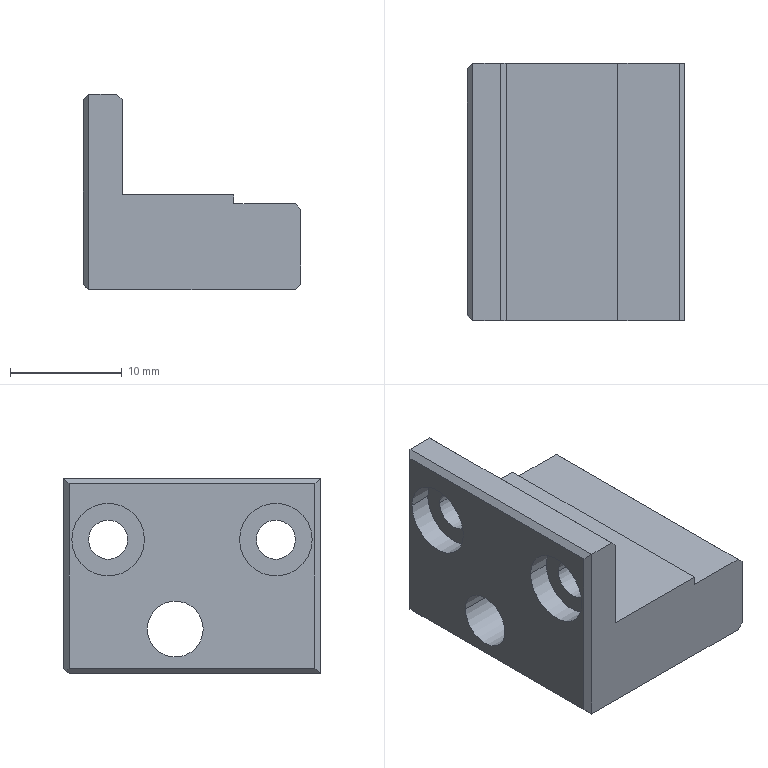Part | NX | 1 solid | 30 faces | box 19.5 x 23 x 17.5 mm | volume 3861 mm3 | plane 20 | cylinder 10 | commonest cylinder face diameters 3.5 x4 6.5 x4 5 x2
STEP:
#1=CARTESIAN_POINT('',(14.,5.5,-9.8));
#2=VERTEX_POINT('',#1);
#3=CARTESIAN_POINT('',(14.,28.5,-9.8));
#4=VERTEX_POINT('',#3);
#5=CARTESIAN_POINT('',(14.,0.,-9.8));
#6=DIRECTION('',(0.,1.,0.));
#7=VECTOR('',#6,1000.);
#8=LINE('',#5,#7);
#9=EDGE_CURVE('',#2,#4,#8,.T.);
#10=ORIENTED_EDGE('',*,*,#9,.F.);
#11=CARTESIAN_POINT('',(19.5,5.5,-9.8));
#12=VERTEX_POINT('',#11);
#13=CARTESIAN_POINT('',(0.,5.5,-9.8));
#14=DIRECTION('',(1.,0.,0.));
#15=VECTOR('',#14,1000.);
#16=LINE('',#13,#15);
#17=EDGE_CURVE('',#2,#12,#16,.T.);
#18=ORIENTED_EDGE('',*,*,#17,.T.);
#19=CARTESIAN_POINT('',(19.5,28.5,-9.8));
#20=VERTEX_POINT('',#19);
#21=CARTESIAN_POINT('',(19.5,14.5,-9.8));
#22=DIRECTION('',(0.,-1.,0.));
#23=VECTOR('',#22,1000.);
#24=LINE('',#21,#23);
#25=EDGE_CURVE('',#20,#12,#24,.T.);
#26=ORIENTED_EDGE('',*,*,#25,.F.);
#27=CARTESIAN_POINT('',(0.,28.5,-9.8));
#28=DIRECTION('',(1.,0.,0.));
#29=VECTOR('',#28,1000.);
#30=LINE('',#27,#29);
#31=EDGE_CURVE('',#4,#20,#30,.T.);
#32=ORIENTED_EDGE('',*,*,#31,.F.);
#33=EDGE_LOOP('',(#10,#18,#26,#32));
#34=FACE_BOUND('',#33,.T.);
#35=CARTESIAN_POINT('',(14.,14.5,-9.8));
#36=DIRECTION('',(0.,0.,1.));
#37=DIRECTION('',(1.,0.,0.));
#38=AXIS2_PLACEMENT_3D('',#35,#36,#37);
#39=PLANE('',#38);
#40=ADVANCED_FACE('',(#34),#39,.T.);
#41=CARTESIAN_POINT('',(2.5,21.25,-5.5));
#42=VERTEX_POINT('',#41);
#43=CARTESIAN_POINT('',(2.5,27.75,-5.5));
#44=VERTEX_POINT('',#43);
#45=CARTESIAN_POINT('',(2.5,24.5,-5.5));
#46=DIRECTION('',(-1.,0.,0.));
#47=DIRECTION('',(0.,1.,0.));
#48=AXIS2_PLACEMENT_3D('',#45,#46,#47);
#49=CIRCLE('',#48,3.25);
#50=EDGE_CURVE('',#42,#44,#49,.T.);
#51=ORIENTED_EDGE('',*,*,#50,.T.);
#52=CARTESIAN_POINT('',(2.5,24.5,-5.5));
#53=DIRECTION('',(-1.,0.,0.));
#54=DIRECTION('',(0.,1.,0.));
#55=AXIS2_PLACEMENT_3D('',#52,#53,#54);
#56=CIRCLE('',#55,3.25);
#57=EDGE_CURVE('',#44,#42,#56,.T.);
#58=ORIENTED_EDGE('',*,*,#57,.T.);
#59=EDGE_LOOP('',(#51,#58));
#60=FACE_BOUND('',#59,.T.);
#61=CARTESIAN_POINT('',(2.5,22.75,-5.5));
#62=VERTEX_POINT('',#61);
#63=CARTESIAN_POINT('',(2.5,26.25,-5.5));
#64=VERTEX_POINT('',#63);
#65=CARTESIAN_POINT('',(2.5,24.5,-5.5));
#66=DIRECTION('',(-1.,0.,0.));
#67=DIRECTION('',(0.,1.,0.));
#68=AXIS2_PLACEMENT_3D('',#65,#66,#67);
#69=CIRCLE('',#68,1.75);
#70=EDGE_CURVE('',#62,#64,#69,.T.);
#71=ORIENTED_EDGE('',*,*,#70,.F.);
#72=CARTESIAN_POINT('',(2.5,24.5,-5.5));
#73=DIRECTION('',(-1.,0.,0.));
#74=DIRECTION('',(0.,1.,0.));
#75=AXIS2_PLACEMENT_3D('',#72,#73,#74);
#76=CIRCLE('',#75,1.75);
#77=EDGE_CURVE('',#64,#62,#76,.T.);
#78=ORIENTED_EDGE('',*,*,#77,.F.);
#79=EDGE_LOOP('',(#71,#78));
#80=FACE_BOUND('',#79,.T.);
#81=CARTESIAN_POINT('',(2.5,24.5,-5.5));
#82=DIRECTION('',(-1.,0.,0.));
#83=DIRECTION('',(0.,0.,1.));
#84=AXIS2_PLACEMENT_3D('',#81,#82,#83);
#85=PLANE('',#84);
#86=ADVANCED_FACE('',(#60,#80),#85,.T.);
#87=CARTESIAN_POINT('',(1.,28.,-17.5));
#88=VERTEX_POINT('',#87);
#89=CARTESIAN_POINT('',(19.5,28.,-17.5));
#90=VERTEX_POINT('',#89);
#91=CARTESIAN_POINT('',(0.,28.,-17.5));
#92=DIRECTION('',(1.,0.,0.));
#93=VECTOR('',#92,1000.);
#94=LINE('',#91,#93);
#95=EDGE_CURVE('',#88,#90,#94,.T.);
#96=ORIENTED_EDGE('',*,*,#95,.F.);
#97=CARTESIAN_POINT('',(0.75,28.25,-17.25));
#98=VERTEX_POINT('',#97);
#99=CARTESIAN_POINT('',(-16.5,45.5,0.));
#100=DIRECTION('',(-0.5774,0.5774,0.5774));
#101=VECTOR('',#100,1000.);
#102=LINE('',#99,#101);
#103=EDGE_CURVE('',#88,#98,#102,.T.);
#104=ORIENTED_EDGE('',*,*,#103,.T.);
#105=CARTESIAN_POINT('',(1.,28.5,-17.));
#106=VERTEX_POINT('',#105);
#107=CARTESIAN_POINT('',(18.,45.5,0.));
#108=DIRECTION('',(-0.5774,-0.5774,-0.5774));
#109=VECTOR('',#108,1000.);
#110=LINE('',#107,#109);
#111=EDGE_CURVE('',#106,#98,#110,.T.);
#112=ORIENTED_EDGE('',*,*,#111,.F.);
#113=CARTESIAN_POINT('',(20.,28.5,-17.));
#114=VERTEX_POINT('',#113);
#115=CARTESIAN_POINT('',(0.,28.5,-17.));
#116=DIRECTION('',(-1.,0.,0.));
#117=VECTOR('',#116,1000.);
#118=LINE('',#115,#117);
#119=EDGE_CURVE('',#114,#106,#118,.T.);
#120=ORIENTED_EDGE('',*,*,#119,.F.);
#121=CARTESIAN_POINT('',(37.,45.5,0.));
#122=DIRECTION('',(0.5774,0.5774,0.5774));
#123=VECTOR('',#122,1000.);
#124=LINE('',#121,#123);
#125=EDGE_CURVE('',#90,#114,#124,.T.);
#126=ORIENTED_EDGE('',*,*,#125,.F.);
#127=EDGE_LOOP('',(#96,#104,#112,#120,#126));
#128=FACE_BOUND('',#127,.T.);
#129=CARTESIAN_POINT('',(7.25,28.25,-17.25));
#130=DIRECTION('',(0.,0.7071,-0.7071));
#131=DIRECTION('',(-1.,0.,0.));
#132=AXIS2_PLACEMENT_3D('',#129,#130,#131);
#133=PLANE('',#132);
#134=ADVANCED_FACE('',(#128),#133,.T.);
#135=CARTESIAN_POINT('',(14.,28.5,-9.));
#136=VERTEX_POINT('',#135);
#137=CARTESIAN_POINT('',(14.,5.5,-9.));
#138=VERTEX_POINT('',#137);
#139=CARTESIAN_POINT('',(14.,0.,-9.));
#140=DIRECTION('',(0.,-1.,0.));
#141=VECTOR('',#140,1000.);
#142=LINE('',#139,#141);
#143=EDGE_CURVE('',#136,#138,#142,.T.);
#144=ORIENTED_EDGE('',*,*,#143,.F.);
#145=CARTESIAN_POINT('',(4.,28.5,-9.));
#146=VERTEX_POINT('',#145);
#147=CARTESIAN_POINT('',(0.,28.5,-9.));
#148=DIRECTION('',(-1.,0.,0.));
#149=VECTOR('',#148,1000.);
#150=LINE('',#147,#149);
#151=EDGE_CURVE('',#136,#146,#150,.T.);
#152=ORIENTED_EDGE('',*,*,#151,.T.);
#153=CARTESIAN_POINT('',(4.,5.5,-9.));
#154=VERTEX_POINT('',#153);
#155=CARTESIAN_POINT('',(4.,0.,-9.));
#156=DIRECTION('',(0.,1.,0.));
#157=VECTOR('',#156,1000.);
#158=LINE('',#155,#157);
#159=EDGE_CURVE('',#154,#146,#158,.T.);
#160=ORIENTED_EDGE('',*,*,#159,.F.);
#161=CARTESIAN_POINT('',(0.,5.5,-9.));
#162=DIRECTION('',(-1.,0.,0.));
#163=VECTOR('',#162,1000.);
#164=LINE('',#161,#163);
#165=EDGE_CURVE('',#138,#154,#164,.T.);
#166=ORIENTED_EDGE('',*,*,#165,.F.);
#167=EDGE_LOOP('',(#144,#152,#160,#166));
#168=FACE_BOUND('',#167,.T.);
#169=CARTESIAN_POINT('',(4.,0.,-9.));
#170=DIRECTION('',(0.,0.,1.));
#171=DIRECTION('',(1.,0.,0.));
#172=AXIS2_PLACEMENT_3D('',#169,#170,#171);
#173=PLANE('',#172);
#174=ADVANCED_FACE('',(#168),#173,.T.);
#175=CARTESIAN_POINT('',(1.,5.5,0.));
#176=VERTEX_POINT('',#175);
#177=CARTESIAN_POINT('',(1.,5.5,-17.5));
#178=VERTEX_POINT('',#177);
#179=CARTESIAN_POINT('',(1.,5.5,0.));
#180=DIRECTION('',(0.,0.,-1.));
#181=VECTOR('',#180,1000.);
#182=LINE('',#179,#181);
#183=EDGE_CURVE('',#176,#178,#182,.T.);
#184=ORIENTED_EDGE('',*,*,#183,.T.);
#185=CARTESIAN_POINT('',(19.5,5.5,-17.5));
#186=VERTEX_POINT('',#185);
#187=CARTESIAN_POINT('',(0.,5.5,-17.5));
#188=DIRECTION('',(-1.,0.,0.));
#189=VECTOR('',#188,1000.);
#190=LINE('',#187,#189);
#191=EDGE_CURVE('',#186,#178,#190,.T.);
#192=ORIENTED_EDGE('',*,*,#191,.F.);
#193=CARTESIAN_POINT('',(20.,5.5,-17.));
#194=VERTEX_POINT('',#193);
#195=CARTESIAN_POINT('',(37.,5.5,0.));
#196=DIRECTION('',(0.7071,0.,0.7071));
#197=VECTOR('',#196,1000.);
#198=LINE('',#195,#197);
#199=EDGE_CURVE('',#186,#194,#198,.T.);
#200=ORIENTED_EDGE('',*,*,#199,.T.);
#201=CARTESIAN_POINT('',(20.,5.5,-10.3));
#202=VERTEX_POINT('',#201);
#203=CARTESIAN_POINT('',(20.,5.5,0.));
#204=DIRECTION('',(0.,0.,1.));
#205=VECTOR('',#204,1000.);
#206=LINE('',#203,#205);
#207=EDGE_CURVE('',#194,#202,#206,.T.);
#208=ORIENTED_EDGE('',*,*,#207,.T.);
#209=CARTESIAN_POINT('',(9.7,5.5,0.));
#210=DIRECTION('',(-0.7071,0.,0.7071));
#211=VECTOR('',#210,1000.);
#212=LINE('',#209,#211);
#213=EDGE_CURVE('',#202,#12,#212,.T.);
#214=ORIENTED_EDGE('',*,*,#213,.T.);
#215=ORIENTED_EDGE('',*,*,#17,.F.);
#216=CARTESIAN_POINT('',(14.,5.5,0.));
#217=DIRECTION('',(0.,0.,-1.));
#218=VECTOR('',#217,1000.);
#219=LINE('',#216,#218);
#220=EDGE_CURVE('',#138,#2,#219,.T.);
#221=ORIENTED_EDGE('',*,*,#220,.F.);
#222=ORIENTED_EDGE('',*,*,#165,.T.);
#223=CARTESIAN_POINT('',(4.,5.5,-0.5));
#224=VERTEX_POINT('',#223);
#225=CARTESIAN_POINT('',(4.,5.5,0.));
#226=DIRECTION('',(0.,0.,1.));
#227=VECTOR('',#226,1000.);
#228=LINE('',#225,#227);
#229=EDGE_CURVE('',#154,#224,#228,.T.);
#230=ORIENTED_EDGE('',*,*,#229,.T.);
#231=CARTESIAN_POINT('',(3.5,5.5,0.));
#232=VERTEX_POINT('',#231);
#233=CARTESIAN_POINT('',(3.5,5.5,0.));
#234=DIRECTION('',(0.7071,0.,-0.7071));
#235=VECTOR('',#234,1000.);
#236=LINE('',#233,#235);
#237=EDGE_CURVE('',#232,#224,#236,.T.);
#238=ORIENTED_EDGE('',*,*,#237,.F.);
#239=CARTESIAN_POINT('',(0.,5.5,0.));
#240=DIRECTION('',(-1.,0.,0.));
#241=VECTOR('',#240,1000.);
#242=LINE('',#239,#241);
#243=EDGE_CURVE('',#232,#176,#242,.T.);
#244=ORIENTED_EDGE('',*,*,#243,.T.);
#245=EDGE_LOOP('',(#184,#192,#200,#208,#214,#215,#221,#222,#230,#238,#244));
#246=FACE_BOUND('',#245,.T.);
#247=CARTESIAN_POINT('',(17.967,5.5,-12.374));
#248=DIRECTION('',(0.,-1.,0.));
#249=DIRECTION('',(0.,0.,-1.));
#250=AXIS2_PLACEMENT_3D('',#247,#248,#249);
#251=PLANE('',#250);
#252=ADVANCED_FACE('',(#246),#251,.T.);
#253=CARTESIAN_POINT('',(1.,28.5,0.));
#254=VERTEX_POINT('',#253);
#255=CARTESIAN_POINT('',(1.,0.,0.));
#256=DIRECTION('',(0.,1.,0.));
#257=VECTOR('',#256,1000.);
#258=LINE('',#255,#257);
#259=EDGE_CURVE('',#176,#254,#258,.T.);
#260=ORIENTED_EDGE('',*,*,#259,.F.);
#261=ORIENTED_EDGE('',*,*,#243,.F.);
#262=CARTESIAN_POINT('',(3.5,28.5,0.));
#263=VERTEX_POINT('',#262);
#264=CARTESIAN_POINT('',(3.5,0.,0.));
#265=DIRECTION('',(0.,1.,0.));
#266=VECTOR('',#265,1000.);
#267=LINE('',#264,#266);
#268=EDGE_CURVE('',#232,#263,#267,.T.);
#269=ORIENTED_EDGE('',*,*,#268,.T.);
#270=CARTESIAN_POINT('',(0.,28.5,0.));
#271=DIRECTION('',(-1.,0.,0.));
#272=VECTOR('',#271,1000.);
#273=LINE('',#270,#272);
#274=EDGE_CURVE('',#263,#254,#273,.T.);
#275=ORIENTED_EDGE('',*,*,#274,.T.);
#276=EDGE_LOOP('',(#260,#261,#269,#275));
#277=FACE_BOUND('',#276,.T.);
#278=CARTESIAN_POINT('',(0.,0.,0.));
#279=DIRECTION('',(0.,0.,1.));
#280=DIRECTION('',(1.,0.,0.));
#281=AXIS2_PLACEMENT_3D('',#278,#279,#280);
#282=PLANE('',#281);
#283=ADVANCED_FACE('',(#277),#282,.T.);
#284=CARTESIAN_POINT('',(20.,28.5,-10.3));
#285=VERTEX_POINT('',#284);
#286=CARTESIAN_POINT('',(20.,0.,-10.3));
#287=DIRECTION('',(0.,1.,0.));
#288=VECTOR('',#287,1000.);
#289=LINE('',#286,#288);
#290=EDGE_CURVE('',#202,#285,#289,.T.);
#291=ORIENTED_EDGE('',*,*,#290,.F.);
#292=ORIENTED_EDGE('',*,*,#207,.F.);
#293=CARTESIAN_POINT('',(20.,0.,-17.));
#294=DIRECTION('',(0.,-1.,0.));
#295=VECTOR('',#294,1000.);
#296=LINE('',#293,#295);
#297=EDGE_CURVE('',#114,#194,#296,.T.);
#298=ORIENTED_EDGE('',*,*,#297,.F.);
#299=CARTESIAN_POINT('',(20.,28.5,0.));
#300=DIRECTION('',(0.,0.,-1.));
#301=VECTOR('',#300,1000.);
#302=LINE('',#299,#301);
#303=EDGE_CURVE('',#285,#114,#302,.T.);
#304=ORIENTED_EDGE('',*,*,#303,.F.);
#305=EDGE_LOOP('',(#291,#292,#298,#304));
#306=FACE_BOUND('',#305,.T.);
#307=CARTESIAN_POINT('',(20.,21.,-13.5));
#308=VERTEX_POINT('',#307);
#309=CARTESIAN_POINT('',(20.,16.,-13.5));
#310=VERTEX_POINT('',#309);
#311=CARTESIAN_POINT('',(20.,18.5,-13.5));
#312=DIRECTION('',(1.,0.,0.));
#313=DIRECTION('',(0.,1.,0.));
#314=AXIS2_PLACEMENT_3D('',#311,#312,#313);
#315=CIRCLE('',#314,2.5);
#316=EDGE_CURVE('',#308,#310,#315,.T.);
#317=ORIENTED_EDGE('',*,*,#316,.F.);
#318=CARTESIAN_POINT('',(20.,18.5,-13.5));
#319=DIRECTION('',(1.,0.,0.));
#320=DIRECTION('',(0.,1.,0.));
#321=AXIS2_PLACEMENT_3D('',#318,#319,#320);
#322=CIRCLE('',#321,2.5);
#323=EDGE_CURVE('',#310,#308,#322,.T.);
#324=ORIENTED_EDGE('',*,*,#323,.F.);
#325=EDGE_LOOP('',(#317,#324));
#326=FACE_BOUND('',#325,.T.);
#327=CARTESIAN_POINT('',(20.,14.5,-10.3));
#328=DIRECTION('',(1.,0.,0.));
#329=DIRECTION('',(0.,1.,0.));
#330=AXIS2_PLACEMENT_3D('',#327,#328,#329);
#331=PLANE('',#330);
#332=ADVANCED_FACE('',(#306,#326),#331,.T.);
#333=ORIENTED_EDGE('',*,*,#119,.T.);
#334=CARTESIAN_POINT('',(1.,28.5,0.));
#335=DIRECTION('',(0.,0.,-1.));
#336=VECTOR('',#335,1000.);
#337=LINE('',#334,#336);
#338=EDGE_CURVE('',#254,#106,#337,.T.);
#339=ORIENTED_EDGE('',*,*,#338,.F.);
#340=ORIENTED_EDGE('',*,*,#274,.F.);
#341=CARTESIAN_POINT('',(4.,28.5,-0.5));
#342=VERTEX_POINT('',#341);
#343=CARTESIAN_POINT('',(3.5,28.5,0.));
#344=DIRECTION('',(0.7071,0.,-0.7071));
#345=VECTOR('',#344,1000.);
#346=LINE('',#343,#345);
#347=EDGE_CURVE('',#263,#342,#346,.T.);
#348=ORIENTED_EDGE('',*,*,#347,.T.);
#349=CARTESIAN_POINT('',(4.,28.5,0.));
#350=DIRECTION('',(0.,0.,1.));
#351=VECTOR('',#350,1000.);
#352=LINE('',#349,#351);
#353=EDGE_CURVE('',#146,#342,#352,.T.);
#354=ORIENTED_EDGE('',*,*,#353,.F.);
#355=ORIENTED_EDGE('',*,*,#151,.F.);
#356=CARTESIAN_POINT('',(14.,28.5,0.));
#357=DIRECTION('',(0.,0.,-1.));
#358=VECTOR('',#357,1000.);
#359=LINE('',#356,#358);
#360=EDGE_CURVE('',#136,#4,#359,.T.);
#361=ORIENTED_EDGE('',*,*,#360,.T.);
#362=ORIENTED_EDGE('',*,*,#31,.T.);
#363=CARTESIAN_POINT('',(9.7,28.5,0.));
#364=DIRECTION('',(0.7071,0.,-0.7071));
#365=VECTOR('',#364,1000.);
#366=LINE('',#363,#365);
#367=EDGE_CURVE('',#20,#285,#366,.T.);
#368=ORIENTED_EDGE('',*,*,#367,.T.);
#369=ORIENTED_EDGE('',*,*,#303,.T.);
#370=EDGE_LOOP('',(#333,#339,#340,#348,#354,#355,#361,#362,#368,#369));
#371=FACE_BOUND('',#370,.T.);
#372=CARTESIAN_POINT('',(0.,28.5,0.));
#373=DIRECTION('',(0.,1.,0.));
#374=DIRECTION('',(1.,0.,0.));
#375=AXIS2_PLACEMENT_3D('',#372,#373,#374);
#376=PLANE('',#375);
#377=ADVANCED_FACE('',(#371),#376,.T.);
#378=CARTESIAN_POINT('',(0.5,6.,-17.));
#379=VERTEX_POINT('',#378);
#380=CARTESIAN_POINT('',(0.5,28.,-17.));
#381=VERTEX_POINT('',#380);
#382=CARTESIAN_POINT('',(0.5,0.,-17.));
#383=DIRECTION('',(0.,1.,0.));
#384=VECTOR('',#383,1000.);
#385=LINE('',#382,#384);
#386=EDGE_CURVE('',#379,#381,#385,.T.);
#387=ORIENTED_EDGE('',*,*,#386,.F.);
#388=CARTESIAN_POINT('',(0.5,6.,-0.5));
#389=VERTEX_POINT('',#388);
#390=CARTESIAN_POINT('',(0.5,6.,0.));
#391=DIRECTION('',(0.,0.,-1.));
#392=VECTOR('',#391,1000.);
#393=LINE('',#390,#392);
#394=EDGE_CURVE('',#389,#379,#393,.T.);
#395=ORIENTED_EDGE('',*,*,#394,.F.);
#396=CARTESIAN_POINT('',(0.5,28.,-0.5));
#397=VERTEX_POINT('',#396);
#398=CARTESIAN_POINT('',(0.5,0.,-0.5));
#399=DIRECTION('',(0.,-1.,0.));
#400=VECTOR('',#399,1000.);
#401=LINE('',#398,#400);
#402=EDGE_CURVE('',#397,#389,#401,.T.);
#403=ORIENTED_EDGE('',*,*,#402,.F.);
#404=CARTESIAN_POINT('',(0.5,28.,0.));
#405=DIRECTION('',(0.,0.,1.));
#406=VECTOR('',#405,1000.);
#407=LINE('',#404,#406);
#408=EDGE_CURVE('',#381,#397,#407,.T.);
#409=ORIENTED_EDGE('',*,*,#408,.F.);
#410=EDGE_LOOP('',(#387,#395,#403,#409));
#411=FACE_BOUND('',#410,.T.);
#412=CARTESIAN_POINT('',(0.5,27.75,-5.5));
#413=VERTEX_POINT('',#412);
#414=CARTESIAN_POINT('',(0.5,21.25,-5.5));
#415=VERTEX_POINT('',#414);
#416=CARTESIAN_POINT('',(0.5,24.5,-5.5));
#417=DIRECTION('',(-1.,0.,0.));
#418=DIRECTION('',(0.,1.,0.));
#419=AXIS2_PLACEMENT_3D('',#416,#417,#418);
#420=CIRCLE('',#419,3.25);
#421=EDGE_CURVE('',#413,#415,#420,.T.);
#422=ORIENTED_EDGE('',*,*,#421,.F.);
#423=CARTESIAN_POINT('',(0.5,24.5,-5.5));
#424=DIRECTION('',(-1.,0.,0.));
#425=DIRECTION('',(0.,1.,0.));
#426=AXIS2_PLACEMENT_3D('',#423,#424,#425);
#427=CIRCLE('',#426,3.25);
#428=EDGE_CURVE('',#415,#413,#427,.T.);
#429=ORIENTED_EDGE('',*,*,#428,.F.);
#430=EDGE_LOOP('',(#422,#429));
#431=FACE_BOUND('',#430,.T.);
#432=CARTESIAN_POINT('',(0.5,16.,-13.5));
#433=VERTEX_POINT('',#432);
#434=CARTESIAN_POINT('',(0.5,21.,-13.5));
#435=VERTEX_POINT('',#434);
#436=CARTESIAN_POINT('',(0.5,18.5,-13.5));
#437=DIRECTION('',(1.,0.,0.));
#438=DIRECTION('',(0.,1.,0.));
#439=AXIS2_PLACEMENT_3D('',#436,#437,#438);
#440=CIRCLE('',#439,2.5);
#441=EDGE_CURVE('',#433,#435,#440,.T.);
#442=ORIENTED_EDGE('',*,*,#441,.T.);
#443=CARTESIAN_POINT('',(0.5,18.5,-13.5));
#444=DIRECTION('',(1.,0.,0.));
#445=DIRECTION('',(0.,1.,0.));
#446=AXIS2_PLACEMENT_3D('',#443,#444,#445);
#447=CIRCLE('',#446,2.5);
#448=EDGE_CURVE('',#435,#433,#447,.T.);
#449=ORIENTED_EDGE('',*,*,#448,.T.);
#450=EDGE_LOOP('',(#442,#449));
#451=FACE_BOUND('',#450,.T.);
#452=CARTESIAN_POINT('',(0.5,12.75,-5.5));
#453=VERTEX_POINT('',#452);
#454=CARTESIAN_POINT('',(0.5,6.25,-5.5));
#455=VERTEX_POINT('',#454);
#456=CARTESIAN_POINT('',(0.5,9.5,-5.5));
#457=DIRECTION('',(-1.,0.,0.));
#458=DIRECTION('',(0.,1.,0.));
#459=AXIS2_PLACEMENT_3D('',#456,#457,#458);
#460=CIRCLE('',#459,3.25);
#461=EDGE_CURVE('',#453,#455,#460,.T.);
#462=ORIENTED_EDGE('',*,*,#461,.F.);
#463=CARTESIAN_POINT('',(0.5,9.5,-5.5));
#464=DIRECTION('',(-1.,0.,0.));
#465=DIRECTION('',(0.,1.,0.));
#466=AXIS2_PLACEMENT_3D('',#463,#464,#465);
#467=CIRCLE('',#466,3.25);
#468=EDGE_CURVE('',#455,#453,#467,.T.);
#469=ORIENTED_EDGE('',*,*,#468,.F.);
#470=EDGE_LOOP('',(#462,#469));
#471=FACE_BOUND('',#470,.T.);
#472=CARTESIAN_POINT('',(0.5,14.5,-17.));
#473=DIRECTION('',(-1.,0.,0.));
#474=DIRECTION('',(0.,0.,1.));
#475=AXIS2_PLACEMENT_3D('',#472,#473,#474);
#476=PLANE('',#475);
#477=ADVANCED_FACE('',(#411,#431,#451,#471),#476,.T.);
#478=ORIENTED_EDGE('',*,*,#259,.T.);
#479=CARTESIAN_POINT('',(1.,28.5,0.));
#480=DIRECTION('',(0.5774,0.5774,0.5774));
#481=VECTOR('',#480,1000.);
#482=LINE('',#479,#481);
#483=EDGE_CURVE('',#397,#254,#482,.T.);
#484=ORIENTED_EDGE('',*,*,#483,.F.);
#485=ORIENTED_EDGE('',*,*,#402,.T.);
#486=CARTESIAN_POINT('',(1.,5.5,0.));
#487=DIRECTION('',(-0.5774,0.5774,-0.5774));
#488=VECTOR('',#487,1000.);
#489=LINE('',#486,#488);
#490=EDGE_CURVE('',#176,#389,#489,.T.);
#491=ORIENTED_EDGE('',*,*,#490,.F.);
#492=EDGE_LOOP('',(#478,#484,#485,#491));
#493=FACE_BOUND('',#492,.T.);
#494=CARTESIAN_POINT('',(0.75,17.,-0.25));
#495=DIRECTION('',(-0.7071,0.,0.7071));
#496=DIRECTION('',(0.,1.,0.));
#497=AXIS2_PLACEMENT_3D('',#494,#495,#496);
#498=PLANE('',#497);
#499=ADVANCED_FACE('',(#493),#498,.T.);
#500=ORIENTED_EDGE('',*,*,#316,.T.);
#501=CARTESIAN_POINT('',(0.,16.,-13.5));
#502=DIRECTION('',(1.,0.,0.));
#503=VECTOR('',#502,1000.);
#504=LINE('',#501,#503);
#505=EDGE_CURVE('',#310,#433,#504,.F.);
#506=ORIENTED_EDGE('',*,*,#505,.T.);
#507=ORIENTED_EDGE('',*,*,#448,.F.);
#508=CARTESIAN_POINT('',(0.,21.,-13.5));
#509=DIRECTION('',(1.,0.,0.));
#510=VECTOR('',#509,1000.);
#511=LINE('',#508,#510);
#512=EDGE_CURVE('',#308,#435,#511,.F.);
#513=ORIENTED_EDGE('',*,*,#512,.F.);
#514=EDGE_LOOP('',(#500,#506,#507,#513));
#515=FACE_BOUND('',#514,.T.);
#516=CARTESIAN_POINT('',(0.,18.5,-13.5));
#517=DIRECTION('',(1.,0.,0.));
#518=DIRECTION('',(0.,1.,0.));
#519=AXIS2_PLACEMENT_3D('',#516,#517,#518);
#520=CYLINDRICAL_SURFACE('',#519,2.5);
#521=ADVANCED_FACE('',(#515),#520,.F.);
#522=CARTESIAN_POINT('',(2.5,6.25,-5.5));
#523=VERTEX_POINT('',#522);
#524=CARTESIAN_POINT('',(2.5,12.75,-5.5));
#525=VERTEX_POINT('',#524);
#526=CARTESIAN_POINT('',(2.5,9.5,-5.5));
#527=DIRECTION('',(-1.,0.,0.));
#528=DIRECTION('',(0.,1.,0.));
#529=AXIS2_PLACEMENT_3D('',#526,#527,#528);
#530=CIRCLE('',#529,3.25);
#531=EDGE_CURVE('',#523,#525,#530,.T.);
#532=ORIENTED_EDGE('',*,*,#531,.T.);
#533=CARTESIAN_POINT('',(2.5,9.5,-5.5));
#534=DIRECTION('',(-1.,0.,0.));
#535=DIRECTION('',(0.,1.,0.));
#536=AXIS2_PLACEMENT_3D('',#533,#534,#535);
#537=CIRCLE('',#536,3.25);
#538=EDGE_CURVE('',#525,#523,#537,.T.);
#539=ORIENTED_EDGE('',*,*,#538,.T.);
#540=EDGE_LOOP('',(#532,#539));
#541=FACE_BOUND('',#540,.T.);
#542=CARTESIAN_POINT('',(2.5,7.75,-5.5));
#543=VERTEX_POINT('',#542);
#544=CARTESIAN_POINT('',(2.5,11.25,-5.5));
#545=VERTEX_POINT('',#544);
#546=CARTESIAN_POINT('',(2.5,9.5,-5.5));
#547=DIRECTION('',(-1.,0.,0.));
#548=DIRECTION('',(0.,1.,0.));
#549=AXIS2_PLACEMENT_3D('',#546,#547,#548);
#550=CIRCLE('',#549,1.75);
#551=EDGE_CURVE('',#543,#545,#550,.T.);
#552=ORIENTED_EDGE('',*,*,#551,.F.);
#553=CARTESIAN_POINT('',(2.5,9.5,-5.5));
#554=DIRECTION('',(-1.,0.,0.));
#555=DIRECTION('',(0.,1.,0.));
#556=AXIS2_PLACEMENT_3D('',#553,#554,#555);
#557=CIRCLE('',#556,1.75);
#558=EDGE_CURVE('',#545,#543,#557,.T.);
#559=ORIENTED_EDGE('',*,*,#558,.F.);
#560=EDGE_LOOP('',(#552,#559));
#561=FACE_BOUND('',#560,.T.);
#562=CARTESIAN_POINT('',(2.5,9.5,-5.5));
#563=DIRECTION('',(-1.,0.,0.));
#564=DIRECTION('',(0.,0.,1.));
#565=AXIS2_PLACEMENT_3D('',#562,#563,#564);
#566=PLANE('',#565);
#567=ADVANCED_FACE('',(#541,#561),#566,.T.);
#568=ORIENTED_EDGE('',*,*,#531,.F.);
#569=CARTESIAN_POINT('',(23.1,6.25,-5.5));
#570=DIRECTION('',(-1.,0.,0.));
#571=VECTOR('',#570,1000.);
#572=LINE('',#569,#571);
#573=EDGE_CURVE('',#455,#523,#572,.F.);
#574=ORIENTED_EDGE('',*,*,#573,.F.);
#575=ORIENTED_EDGE('',*,*,#468,.T.);
#576=CARTESIAN_POINT('',(23.1,12.75,-5.5));
#577=DIRECTION('',(-1.,0.,0.));
#578=VECTOR('',#577,1000.);
#579=LINE('',#576,#578);
#580=EDGE_CURVE('',#453,#525,#579,.F.);
#581=ORIENTED_EDGE('',*,*,#580,.T.);
#582=EDGE_LOOP('',(#568,#574,#575,#581));
#583=FACE_BOUND('',#582,.T.);
#584=CARTESIAN_POINT('',(23.1,9.5,-5.5));
#585=DIRECTION('',(-1.,0.,0.));
#586=DIRECTION('',(0.,1.,0.));
#587=AXIS2_PLACEMENT_3D('',#584,#585,#586);
#588=CYLINDRICAL_SURFACE('',#587,3.25);
#589=ADVANCED_FACE('',(#583),#588,.F.);
#590=CARTESIAN_POINT('',(4.,26.25,-5.5));
#591=VERTEX_POINT('',#590);
#592=CARTESIAN_POINT('',(4.,22.75,-5.5));
#593=VERTEX_POINT('',#592);
#594=CARTESIAN_POINT('',(4.,24.5,-5.5));
#595=DIRECTION('',(-1.,0.,0.));
#596=DIRECTION('',(0.,1.,0.));
#597=AXIS2_PLACEMENT_3D('',#594,#595,#596);
#598=CIRCLE('',#597,1.75);
#599=EDGE_CURVE('',#591,#593,#598,.T.);
#600=ORIENTED_EDGE('',*,*,#599,.F.);
#601=CARTESIAN_POINT('',(23.1,26.25,-5.5));
#602=DIRECTION('',(-1.,0.,0.));
#603=VECTOR('',#602,1000.);
#604=LINE('',#601,#603);
#605=EDGE_CURVE('',#591,#64,#604,.T.);
#606=ORIENTED_EDGE('',*,*,#605,.T.);
#607=ORIENTED_EDGE('',*,*,#77,.T.);
#608=CARTESIAN_POINT('',(23.1,22.75,-5.5));
#609=DIRECTION('',(-1.,0.,0.));
#610=VECTOR('',#609,1000.);
#611=LINE('',#608,#610);
#612=EDGE_CURVE('',#593,#62,#611,.T.);
#613=ORIENTED_EDGE('',*,*,#612,.F.);
#614=EDGE_LOOP('',(#600,#606,#607,#613));
#615=FACE_BOUND('',#614,.T.);
#616=CARTESIAN_POINT('',(23.1,24.5,-5.5));
#617=DIRECTION('',(-1.,0.,0.));
#618=DIRECTION('',(0.,1.,0.));
#619=AXIS2_PLACEMENT_3D('',#616,#617,#618);
#620=CYLINDRICAL_SURFACE('',#619,1.75);
#621=ADVANCED_FACE('',(#615),#620,.F.);
#622=CARTESIAN_POINT('',(4.,0.,-0.5));
#623=DIRECTION('',(0.,-1.,0.));
#624=VECTOR('',#623,1000.);
#625=LINE('',#622,#624);
#626=EDGE_CURVE('',#342,#224,#625,.T.);
#627=ORIENTED_EDGE('',*,*,#626,.T.);
#628=ORIENTED_EDGE('',*,*,#229,.F.);
#629=ORIENTED_EDGE('',*,*,#159,.T.);
#630=ORIENTED_EDGE('',*,*,#353,.T.);
#631=EDGE_LOOP('',(#627,#628,#629,#630));
#632=FACE_BOUND('',#631,.T.);
#633=CARTESIAN_POINT('',(4.,7.75,-5.5));
#634=VERTEX_POINT('',#633);
#635=CARTESIAN_POINT('',(4.,11.25,-5.5));
#636=VERTEX_POINT('',#635);
#637=CARTESIAN_POINT('',(4.,9.5,-5.5));
#638=DIRECTION('',(-1.,0.,0.));
#639=DIRECTION('',(0.,1.,0.));
#640=AXIS2_PLACEMENT_3D('',#637,#638,#639);
#641=CIRCLE('',#640,1.75);
#642=EDGE_CURVE('',#634,#636,#641,.T.);
#643=ORIENTED_EDGE('',*,*,#642,.T.);
#644=CARTESIAN_POINT('',(4.,9.5,-5.5));
#645=DIRECTION('',(-1.,0.,0.));
#646=DIRECTION('',(0.,1.,0.));
#647=AXIS2_PLACEMENT_3D('',#644,#645,#646);
#648=CIRCLE('',#647,1.75);
#649=EDGE_CURVE('',#636,#634,#648,.T.);
#650=ORIENTED_EDGE('',*,*,#649,.T.);
#651=EDGE_LOOP('',(#643,#650));
#652=FACE_BOUND('',#651,.T.);
#653=ORIENTED_EDGE('',*,*,#599,.T.);
#654=CARTESIAN_POINT('',(4.,24.5,-5.5));
#655=DIRECTION('',(-1.,0.,0.));
#656=DIRECTION('',(0.,1.,0.));
#657=AXIS2_PLACEMENT_3D('',#654,#655,#656);
#658=CIRCLE('',#657,1.75);
#659=EDGE_CURVE('',#593,#591,#658,.T.);
#660=ORIENTED_EDGE('',*,*,#659,.T.);
#661=EDGE_LOOP('',(#653,#660));
#662=FACE_BOUND('',#661,.T.);
#663=CARTESIAN_POINT('',(4.,0.,0.));
#664=DIRECTION('',(1.,0.,0.));
#665=DIRECTION('',(0.,1.,0.));
#666=AXIS2_PLACEMENT_3D('',#663,#664,#665);
#667=PLANE('',#666);
#668=ADVANCED_FACE('',(#632,#652,#662),#667,.T.);
#669=ORIENTED_EDGE('',*,*,#642,.F.);
#670=CARTESIAN_POINT('',(23.1,7.75,-5.5));
#671=DIRECTION('',(-1.,0.,0.));
#672=VECTOR('',#671,1000.);
#673=LINE('',#670,#672);
#674=EDGE_CURVE('',#634,#543,#673,.T.);
#675=ORIENTED_EDGE('',*,*,#674,.T.);
#676=ORIENTED_EDGE('',*,*,#551,.T.);
#677=CARTESIAN_POINT('',(23.1,11.25,-5.5));
#678=DIRECTION('',(-1.,0.,0.));
#679=VECTOR('',#678,1000.);
#680=LINE('',#677,#679);
#681=EDGE_CURVE('',#636,#545,#680,.T.);
#682=ORIENTED_EDGE('',*,*,#681,.F.);
#683=EDGE_LOOP('',(#669,#675,#676,#682));
#684=FACE_BOUND('',#683,.T.);
#685=CARTESIAN_POINT('',(23.1,9.5,-5.5));
#686=DIRECTION('',(-1.,0.,0.));
#687=DIRECTION('',(0.,1.,0.));
#688=AXIS2_PLACEMENT_3D('',#685,#686,#687);
#689=CYLINDRICAL_SURFACE('',#688,1.75);
#690=ADVANCED_FACE('',(#684),#689,.F.);
#691=ORIENTED_EDGE('',*,*,#50,.F.);
#692=CARTESIAN_POINT('',(23.1,21.25,-5.5));
#693=DIRECTION('',(-1.,0.,0.));
#694=VECTOR('',#693,1000.);
#695=LINE('',#692,#694);
#696=EDGE_CURVE('',#415,#42,#695,.F.);
#697=ORIENTED_EDGE('',*,*,#696,.F.);
#698=ORIENTED_EDGE('',*,*,#428,.T.);
#699=CARTESIAN_POINT('',(23.1,27.75,-5.5));
#700=DIRECTION('',(-1.,0.,0.));
#701=VECTOR('',#700,1000.);
#702=LINE('',#699,#701);
#703=EDGE_CURVE('',#413,#44,#702,.F.);
#704=ORIENTED_EDGE('',*,*,#703,.T.);
#705=EDGE_LOOP('',(#691,#697,#698,#704));
#706=FACE_BOUND('',#705,.T.);
#707=CARTESIAN_POINT('',(23.1,24.5,-5.5));
#708=DIRECTION('',(-1.,0.,0.));
#709=DIRECTION('',(0.,1.,0.));
#710=AXIS2_PLACEMENT_3D('',#707,#708,#709);
#711=CYLINDRICAL_SURFACE('',#710,3.25);
#712=ADVANCED_FACE('',(#706),#711,.F.);
#713=ORIENTED_EDGE('',*,*,#297,.T.);
#714=ORIENTED_EDGE('',*,*,#199,.F.);
#715=CARTESIAN_POINT('',(19.5,24.,-17.5));
#716=DIRECTION('',(0.,1.,0.));
#717=VECTOR('',#716,1000.);
#718=LINE('',#715,#717);
#719=EDGE_CURVE('',#186,#90,#718,.T.);
#720=ORIENTED_EDGE('',*,*,#719,.T.);
#721=ORIENTED_EDGE('',*,*,#125,.T.);
#722=EDGE_LOOP('',(#713,#714,#720,#721));
#723=FACE_BOUND('',#722,.T.);
#724=CARTESIAN_POINT('',(20.,14.5,-17.));
#725=DIRECTION('',(0.7071,0.,-0.7071));
#726=DIRECTION('',(0.,-1.,0.));
#727=AXIS2_PLACEMENT_3D('',#724,#725,#726);
#728=PLANE('',#727);
#729=ADVANCED_FACE('',(#723),#728,.T.);
#730=CARTESIAN_POINT('',(1.,14.5,-17.5));
#731=DIRECTION('',(0.,-1.,0.));
#732=VECTOR('',#731,1000.);
#733=LINE('',#730,#732);
#734=EDGE_CURVE('',#88,#178,#733,.T.);
#735=ORIENTED_EDGE('',*,*,#734,.T.);
#736=CARTESIAN_POINT('',(6.5,0.,-23.));
#737=DIRECTION('',(-0.5774,0.5774,0.5774));
#738=VECTOR('',#737,1000.);
#739=LINE('',#736,#738);
#740=EDGE_CURVE('',#178,#379,#739,.T.);
#741=ORIENTED_EDGE('',*,*,#740,.T.);
#742=ORIENTED_EDGE('',*,*,#386,.T.);
#743=CARTESIAN_POINT('',(-16.5,11.,0.));
#744=DIRECTION('',(0.5774,0.5774,-0.5774));
#745=VECTOR('',#744,1000.);
#746=LINE('',#743,#745);
#747=EDGE_CURVE('',#381,#98,#746,.T.);
#748=ORIENTED_EDGE('',*,*,#747,.T.);
#749=ORIENTED_EDGE('',*,*,#103,.F.);
#750=EDGE_LOOP('',(#735,#741,#742,#748,#749));
#751=FACE_BOUND('',#750,.T.);
#752=CARTESIAN_POINT('',(1.,14.5,-17.5));
#753=DIRECTION('',(-0.7071,0.,-0.7071));
#754=DIRECTION('',(-0.7071,0.,0.7071));
#755=AXIS2_PLACEMENT_3D('',#752,#753,#754);
#756=PLANE('',#755);
#757=ADVANCED_FACE('',(#751),#756,.T.);
#758=ORIENTED_EDGE('',*,*,#338,.T.);
#759=ORIENTED_EDGE('',*,*,#111,.T.);
#760=ORIENTED_EDGE('',*,*,#747,.F.);
#761=ORIENTED_EDGE('',*,*,#408,.T.);
#762=ORIENTED_EDGE('',*,*,#483,.T.);
#763=EDGE_LOOP('',(#758,#759,#760,#761,#762));
#764=FACE_BOUND('',#763,.T.);
#765=CARTESIAN_POINT('',(0.75,28.25,-8.5));
#766=DIRECTION('',(-0.7071,0.7071,0.));
#767=DIRECTION('',(0.,0.,1.));
#768=AXIS2_PLACEMENT_3D('',#765,#766,#767);
#769=PLANE('',#768);
#770=ADVANCED_FACE('',(#764),#769,.T.);
#771=ORIENTED_EDGE('',*,*,#9,.T.);
#772=ORIENTED_EDGE('',*,*,#360,.F.);
#773=ORIENTED_EDGE('',*,*,#143,.T.);
#774=ORIENTED_EDGE('',*,*,#220,.T.);
#775=EDGE_LOOP('',(#771,#772,#773,#774));
#776=FACE_BOUND('',#775,.T.);
#777=CARTESIAN_POINT('',(14.,26.,-19.25));
#778=DIRECTION('',(-1.,0.,0.));
#779=DIRECTION('',(0.,0.,1.));
#780=AXIS2_PLACEMENT_3D('',#777,#778,#779);
#781=PLANE('',#780);
#782=ADVANCED_FACE('',(#776),#781,.F.);
#783=ORIENTED_EDGE('',*,*,#626,.F.);
#784=ORIENTED_EDGE('',*,*,#347,.F.);
#785=ORIENTED_EDGE('',*,*,#268,.F.);
#786=ORIENTED_EDGE('',*,*,#237,.T.);
#787=EDGE_LOOP('',(#783,#784,#785,#786));
#788=FACE_BOUND('',#787,.T.);
#789=CARTESIAN_POINT('',(3.75,17.,-0.25));
#790=DIRECTION('',(-0.7071,0.,-0.7071));
#791=DIRECTION('',(-0.7071,0.,0.7071));
#792=AXIS2_PLACEMENT_3D('',#789,#790,#791);
#793=PLANE('',#792);
#794=ADVANCED_FACE('',(#788),#793,.F.);
#795=ORIENTED_EDGE('',*,*,#25,.T.);
#796=ORIENTED_EDGE('',*,*,#213,.F.);
#797=ORIENTED_EDGE('',*,*,#290,.T.);
#798=ORIENTED_EDGE('',*,*,#367,.F.);
#799=EDGE_LOOP('',(#795,#796,#797,#798));
#800=FACE_BOUND('',#799,.T.);
#801=CARTESIAN_POINT('',(19.75,19.25,-10.05));
#802=DIRECTION('',(0.7071,0.,0.7071));
#803=DIRECTION('',(0.,-1.,0.));
#804=AXIS2_PLACEMENT_3D('',#801,#802,#803);
#805=PLANE('',#804);
#806=ADVANCED_FACE('',(#800),#805,.T.);
#807=ORIENTED_EDGE('',*,*,#719,.F.);
#808=ORIENTED_EDGE('',*,*,#191,.T.);
#809=ORIENTED_EDGE('',*,*,#734,.F.);
#810=ORIENTED_EDGE('',*,*,#95,.T.);
#811=EDGE_LOOP('',(#807,#808,#809,#810));
#812=FACE_BOUND('',#811,.T.);
#813=CARTESIAN_POINT('',(19.5,14.5,-17.5));
#814=DIRECTION('',(0.,0.,-1.));
#815=DIRECTION('',(0.,-1.,0.));
#816=AXIS2_PLACEMENT_3D('',#813,#814,#815);
#817=PLANE('',#816);
#818=ADVANCED_FACE('',(#812),#817,.T.);
#819=ORIENTED_EDGE('',*,*,#394,.T.);
#820=ORIENTED_EDGE('',*,*,#740,.F.);
#821=ORIENTED_EDGE('',*,*,#183,.F.);
#822=ORIENTED_EDGE('',*,*,#490,.T.);
#823=EDGE_LOOP('',(#819,#820,#821,#822));
#824=FACE_BOUND('',#823,.T.);
#825=CARTESIAN_POINT('',(0.75,5.75,-6.25));
#826=DIRECTION('',(-0.7071,-0.7071,0.));
#827=DIRECTION('',(-0.7071,0.7071,0.));
#828=AXIS2_PLACEMENT_3D('',#825,#826,#827);
#829=PLANE('',#828);
#830=ADVANCED_FACE('',(#824),#829,.T.);
#831=ORIENTED_EDGE('',*,*,#441,.F.);
#832=ORIENTED_EDGE('',*,*,#505,.F.);
#833=ORIENTED_EDGE('',*,*,#323,.T.);
#834=ORIENTED_EDGE('',*,*,#512,.T.);
#835=EDGE_LOOP('',(#831,#832,#833,#834));
#836=FACE_BOUND('',#835,.T.);
#837=CARTESIAN_POINT('',(0.,18.5,-13.5));
#838=DIRECTION('',(1.,0.,0.));
#839=DIRECTION('',(0.,1.,0.));
#840=AXIS2_PLACEMENT_3D('',#837,#838,#839);
#841=CYLINDRICAL_SURFACE('',#840,2.5);
#842=ADVANCED_FACE('',(#836),#841,.F.);
#843=ORIENTED_EDGE('',*,*,#421,.T.);
#844=ORIENTED_EDGE('',*,*,#696,.T.);
#845=ORIENTED_EDGE('',*,*,#57,.F.);
#846=ORIENTED_EDGE('',*,*,#703,.F.);
#847=EDGE_LOOP('',(#843,#844,#845,#846));
#848=FACE_BOUND('',#847,.T.);
#849=CARTESIAN_POINT('',(23.1,24.5,-5.5));
#850=DIRECTION('',(-1.,0.,0.));
#851=DIRECTION('',(0.,1.,0.));
#852=AXIS2_PLACEMENT_3D('',#849,#850,#851);
#853=CYLINDRICAL_SURFACE('',#852,3.25);
#854=ADVANCED_FACE('',(#848),#853,.F.);
#855=ORIENTED_EDGE('',*,*,#461,.T.);
#856=ORIENTED_EDGE('',*,*,#573,.T.);
#857=ORIENTED_EDGE('',*,*,#538,.F.);
#858=ORIENTED_EDGE('',*,*,#580,.F.);
#859=EDGE_LOOP('',(#855,#856,#857,#858));
#860=FACE_BOUND('',#859,.T.);
#861=CARTESIAN_POINT('',(23.1,9.5,-5.5));
#862=DIRECTION('',(-1.,0.,0.));
#863=DIRECTION('',(0.,1.,0.));
#864=AXIS2_PLACEMENT_3D('',#861,#862,#863);
#865=CYLINDRICAL_SURFACE('',#864,3.25);
#866=ADVANCED_FACE('',(#860),#865,.F.);
#867=ORIENTED_EDGE('',*,*,#681,.T.);
#868=ORIENTED_EDGE('',*,*,#558,.T.);
#869=ORIENTED_EDGE('',*,*,#674,.F.);
#870=ORIENTED_EDGE('',*,*,#649,.F.);
#871=EDGE_LOOP('',(#867,#868,#869,#870));
#872=FACE_BOUND('',#871,.T.);
#873=CARTESIAN_POINT('',(23.1,9.5,-5.5));
#874=DIRECTION('',(-1.,0.,0.));
#875=DIRECTION('',(0.,1.,0.));
#876=AXIS2_PLACEMENT_3D('',#873,#874,#875);
#877=CYLINDRICAL_SURFACE('',#876,1.75);
#878=ADVANCED_FACE('',(#872),#877,.F.);
#879=ORIENTED_EDGE('',*,*,#70,.T.);
#880=ORIENTED_EDGE('',*,*,#605,.F.);
#881=ORIENTED_EDGE('',*,*,#659,.F.);
#882=ORIENTED_EDGE('',*,*,#612,.T.);
#883=EDGE_LOOP('',(#879,#880,#881,#882));
#884=FACE_BOUND('',#883,.T.);
#885=CARTESIAN_POINT('',(23.1,24.5,-5.5));
#886=DIRECTION('',(-1.,0.,0.));
#887=DIRECTION('',(0.,1.,0.));
#888=AXIS2_PLACEMENT_3D('',#885,#886,#887);
#889=CYLINDRICAL_SURFACE('',#888,1.75);
#890=ADVANCED_FACE('',(#884),#889,.F.);
#891=CLOSED_SHELL('',(#40,#86,#134,#174,#252,#283,#332,#377,#477,#499,#521,#567,#589,#621,#668,#690,#712,#729,#757,#770,#782,#794,#806,#818,#830,#842,#854,#866,#878,#890));
#892=MANIFOLD_SOLID_BREP('',#891);
#893=(LENGTH_UNIT()NAMED_UNIT(*)SI_UNIT(.MILLI.,.METRE.));
#894=UNCERTAINTY_MEASURE_WITH_UNIT(LENGTH_MEASURE(0.00001),#893,'','');
#895=(NAMED_UNIT(*)PLANE_ANGLE_UNIT()SI_UNIT($,.RADIAN.));
#896=(NAMED_UNIT(*)SI_UNIT($,.STERADIAN.)SOLID_ANGLE_UNIT());
#897=(GEOMETRIC_REPRESENTATION_CONTEXT(3)GLOBAL_UNCERTAINTY_ASSIGNED_CONTEXT((#894))GLOBAL_UNIT_ASSIGNED_CONTEXT((#893,#895,#896))REPRESENTATION_CONTEXT('',''));
#898=ADVANCED_BREP_SHAPE_REPRESENTATION('',(#892),#897);